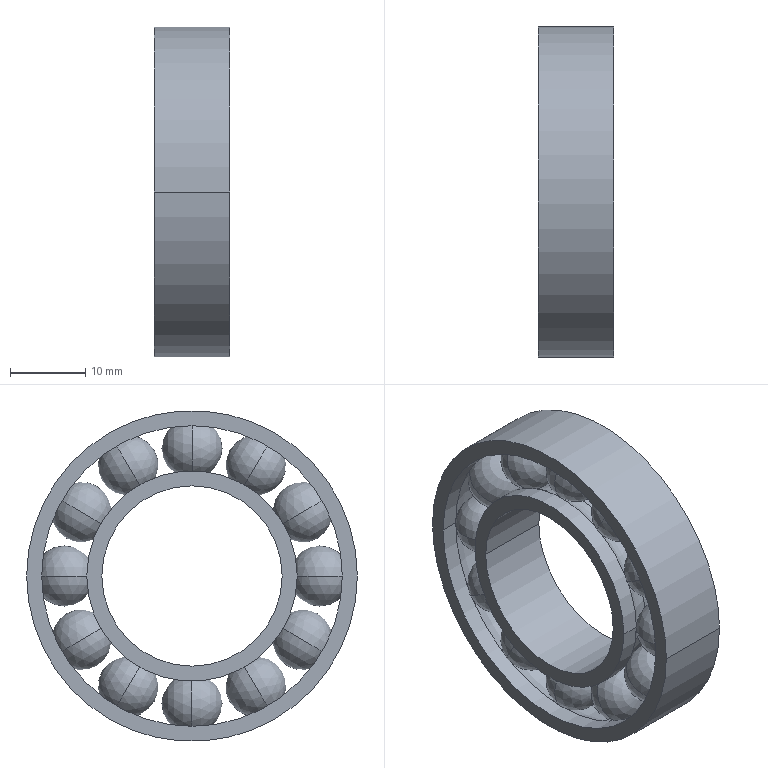Part | SolidWorks | features SavedExtBody 14 | 14 solids | 46 faces | box 10 x 44 x 44 mm | volume 6715 mm3 | sphere 24 | cylinder 12 | torus 6 | plane 4 | commonest cylinder face diameters 28 x4 40 x4 24 x2 44 x2
STEP:
#1=CARTESIAN_POINT('',(-83.272,6.5,53.742));
#2=VERTEX_POINT('',#1);
#3=CARTESIAN_POINT('',(-83.272,10.5,46.813));
#4=VERTEX_POINT('',#3);
#5=CARTESIAN_POINT('',(-83.272,8.5,50.278));
#6=DIRECTION('',(0.,0.866,0.5));
#7=DIRECTION('',(0.,-0.5,0.866));
#8=AXIS2_PLACEMENT_3D('',#5,#6,#7);
#9=CIRCLE('',#8,4.);
#10=EDGE_CURVE('',#2,#4,#9,.T.);
#11=ORIENTED_EDGE('',*,*,#10,.F.);
#12=CARTESIAN_POINT('',(-83.272,8.5,50.278));
#13=DIRECTION('',(0.,-0.866,-0.5));
#14=DIRECTION('',(0.,0.5,-0.866));
#15=AXIS2_PLACEMENT_3D('',#12,#13,#14);
#16=CIRCLE('',#15,4.);
#17=EDGE_CURVE('',#2,#4,#16,.T.);
#18=ORIENTED_EDGE('',*,*,#17,.T.);
#19=EDGE_LOOP('',(#11,#18));
#20=FACE_OUTER_BOUND('',#19,.T.);
#21=CARTESIAN_POINT('',(-83.272,8.5,50.278));
#22=DIRECTION('',(0.,-0.866,-0.5));
#23=DIRECTION('',(1.,0.,0.));
#24=AXIS2_PLACEMENT_3D('',#21,#22,#23);
#25=SPHERICAL_SURFACE('',#24,4.);
#26=ADVANCED_FACE('',(#20),#25,.T.);
#27=ORIENTED_EDGE('',*,*,#17,.F.);
#28=ORIENTED_EDGE('',*,*,#10,.T.);
#29=EDGE_LOOP('',(#27,#28));
#30=FACE_OUTER_BOUND('',#29,.T.);
#31=CARTESIAN_POINT('',(-83.272,8.5,50.278));
#32=DIRECTION('',(0.,-0.866,-0.5));
#33=DIRECTION('',(1.,0.,0.));
#34=AXIS2_PLACEMENT_3D('',#31,#32,#33);
#35=SPHERICAL_SURFACE('',#34,4.);
#36=ADVANCED_FACE('',(#30),#35,.T.);
#37=CLOSED_SHELL('',(#26,#36));
#38=MANIFOLD_SOLID_BREP('',#37);
#39=CARTESIAN_POINT('',(-83.272,11.258,58.5));
#40=VERTEX_POINT('',#39);
#41=CARTESIAN_POINT('',(-83.272,18.187,54.5));
#42=VERTEX_POINT('',#41);
#43=CARTESIAN_POINT('',(-83.272,14.722,56.5));
#44=DIRECTION('',(0.,0.5,0.866));
#45=DIRECTION('',(0.,-0.866,0.5));
#46=AXIS2_PLACEMENT_3D('',#43,#44,#45);
#47=CIRCLE('',#46,4.);
#48=EDGE_CURVE('',#40,#42,#47,.T.);
#49=ORIENTED_EDGE('',*,*,#48,.F.);
#50=CARTESIAN_POINT('',(-83.272,14.722,56.5));
#51=DIRECTION('',(0.,-0.5,-0.866));
#52=DIRECTION('',(0.,0.866,-0.5));
#53=AXIS2_PLACEMENT_3D('',#50,#51,#52);
#54=CIRCLE('',#53,4.);
#55=EDGE_CURVE('',#40,#42,#54,.T.);
#56=ORIENTED_EDGE('',*,*,#55,.T.);
#57=EDGE_LOOP('',(#49,#56));
#58=FACE_OUTER_BOUND('',#57,.T.);
#59=CARTESIAN_POINT('',(-83.272,14.722,56.5));
#60=DIRECTION('',(0.,-0.5,-0.866));
#61=DIRECTION('',(1.,0.,0.));
#62=AXIS2_PLACEMENT_3D('',#59,#60,#61);
#63=SPHERICAL_SURFACE('',#62,4.);
#64=ADVANCED_FACE('',(#58),#63,.T.);
#65=ORIENTED_EDGE('',*,*,#55,.F.);
#66=ORIENTED_EDGE('',*,*,#48,.T.);
#67=EDGE_LOOP('',(#65,#66));
#68=FACE_OUTER_BOUND('',#67,.T.);
#69=CARTESIAN_POINT('',(-83.272,14.722,56.5));
#70=DIRECTION('',(0.,-0.5,-0.866));
#71=DIRECTION('',(1.,0.,0.));
#72=AXIS2_PLACEMENT_3D('',#69,#70,#71);
#73=SPHERICAL_SURFACE('',#72,4.);
#74=ADVANCED_FACE('',(#68),#73,.T.);
#75=CLOSED_SHELL('',(#64,#74));
#76=MANIFOLD_SOLID_BREP('',#75);
#77=CARTESIAN_POINT('',(-83.272,13.,65.));
#78=VERTEX_POINT('',#77);
#79=CARTESIAN_POINT('',(-83.272,21.,65.));
#80=VERTEX_POINT('',#79);
#81=CARTESIAN_POINT('',(-83.272,17.,65.));
#82=DIRECTION('',(0.,0.,1.));
#83=DIRECTION('',(1.,0.,0.));
#84=AXIS2_PLACEMENT_3D('',#81,#82,#83);
#85=CIRCLE('',#84,4.);
#86=EDGE_CURVE('',#78,#80,#85,.T.);
#87=ORIENTED_EDGE('',*,*,#86,.F.);
#88=CARTESIAN_POINT('',(-83.272,17.,65.));
#89=DIRECTION('',(0.,0.,-1.));
#90=DIRECTION('',(-1.,0.,0.));
#91=AXIS2_PLACEMENT_3D('',#88,#89,#90);
#92=CIRCLE('',#91,4.);
#93=EDGE_CURVE('',#78,#80,#92,.T.);
#94=ORIENTED_EDGE('',*,*,#93,.T.);
#95=EDGE_LOOP('',(#87,#94));
#96=FACE_OUTER_BOUND('',#95,.T.);
#97=CARTESIAN_POINT('',(-83.272,17.,65.));
#98=DIRECTION('',(0.,0.,-1.));
#99=DIRECTION('',(1.,0.,0.));
#100=AXIS2_PLACEMENT_3D('',#97,#98,#99);
#101=SPHERICAL_SURFACE('',#100,4.);
#102=ADVANCED_FACE('',(#96),#101,.T.);
#103=ORIENTED_EDGE('',*,*,#93,.F.);
#104=ORIENTED_EDGE('',*,*,#86,.T.);
#105=EDGE_LOOP('',(#103,#104));
#106=FACE_OUTER_BOUND('',#105,.T.);
#107=CARTESIAN_POINT('',(-83.272,17.,65.));
#108=DIRECTION('',(0.,0.,-1.));
#109=DIRECTION('',(1.,0.,0.));
#110=AXIS2_PLACEMENT_3D('',#107,#108,#109);
#111=SPHERICAL_SURFACE('',#110,4.);
#112=ADVANCED_FACE('',(#106),#111,.T.);
#113=CLOSED_SHELL('',(#102,#112));
#114=MANIFOLD_SOLID_BREP('',#113);
#115=CARTESIAN_POINT('',(-83.272,11.258,71.5));
#116=VERTEX_POINT('',#115);
#117=CARTESIAN_POINT('',(-83.272,18.187,75.5));
#118=VERTEX_POINT('',#117);
#119=CARTESIAN_POINT('',(-83.272,14.722,73.5));
#120=DIRECTION('',(0.,-0.5,0.866));
#121=DIRECTION('',(0.,-0.866,-0.5));
#122=AXIS2_PLACEMENT_3D('',#119,#120,#121);
#123=CIRCLE('',#122,4.);
#124=EDGE_CURVE('',#116,#118,#123,.T.);
#125=ORIENTED_EDGE('',*,*,#124,.F.);
#126=CARTESIAN_POINT('',(-83.272,14.722,73.5));
#127=DIRECTION('',(0.,0.5,-0.866));
#128=DIRECTION('',(0.,0.866,0.5));
#129=AXIS2_PLACEMENT_3D('',#126,#127,#128);
#130=CIRCLE('',#129,4.);
#131=EDGE_CURVE('',#116,#118,#130,.T.);
#132=ORIENTED_EDGE('',*,*,#131,.T.);
#133=EDGE_LOOP('',(#125,#132));
#134=FACE_OUTER_BOUND('',#133,.T.);
#135=CARTESIAN_POINT('',(-83.272,14.722,73.5));
#136=DIRECTION('',(0.,0.5,-0.866));
#137=DIRECTION('',(1.,0.,0.));
#138=AXIS2_PLACEMENT_3D('',#135,#136,#137);
#139=SPHERICAL_SURFACE('',#138,4.);
#140=ADVANCED_FACE('',(#134),#139,.T.);
#141=ORIENTED_EDGE('',*,*,#131,.F.);
#142=ORIENTED_EDGE('',*,*,#124,.T.);
#143=EDGE_LOOP('',(#141,#142));
#144=FACE_OUTER_BOUND('',#143,.T.);
#145=CARTESIAN_POINT('',(-83.272,14.722,73.5));
#146=DIRECTION('',(0.,0.5,-0.866));
#147=DIRECTION('',(1.,0.,0.));
#148=AXIS2_PLACEMENT_3D('',#145,#146,#147);
#149=SPHERICAL_SURFACE('',#148,4.);
#150=ADVANCED_FACE('',(#144),#149,.T.);
#151=CLOSED_SHELL('',(#140,#150));
#152=MANIFOLD_SOLID_BREP('',#151);
#153=CARTESIAN_POINT('',(-83.272,6.5,76.258));
#154=VERTEX_POINT('',#153);
#155=CARTESIAN_POINT('',(-83.272,10.5,83.187));
#156=VERTEX_POINT('',#155);
#157=CARTESIAN_POINT('',(-83.272,8.5,79.722));
#158=DIRECTION('',(0.,-0.866,0.5));
#159=DIRECTION('',(0.,-0.5,-0.866));
#160=AXIS2_PLACEMENT_3D('',#157,#158,#159);
#161=CIRCLE('',#160,4.);
#162=EDGE_CURVE('',#154,#156,#161,.T.);
#163=ORIENTED_EDGE('',*,*,#162,.F.);
#164=CARTESIAN_POINT('',(-83.272,8.5,79.722));
#165=DIRECTION('',(0.,0.866,-0.5));
#166=DIRECTION('',(0.,0.5,0.866));
#167=AXIS2_PLACEMENT_3D('',#164,#165,#166);
#168=CIRCLE('',#167,4.);
#169=EDGE_CURVE('',#154,#156,#168,.T.);
#170=ORIENTED_EDGE('',*,*,#169,.T.);
#171=EDGE_LOOP('',(#163,#170));
#172=FACE_OUTER_BOUND('',#171,.T.);
#173=CARTESIAN_POINT('',(-83.272,8.5,79.722));
#174=DIRECTION('',(0.,0.866,-0.5));
#175=DIRECTION('',(1.,0.,0.));
#176=AXIS2_PLACEMENT_3D('',#173,#174,#175);
#177=SPHERICAL_SURFACE('',#176,4.);
#178=ADVANCED_FACE('',(#172),#177,.T.);
#179=ORIENTED_EDGE('',*,*,#169,.F.);
#180=ORIENTED_EDGE('',*,*,#162,.T.);
#181=EDGE_LOOP('',(#179,#180));
#182=FACE_OUTER_BOUND('',#181,.T.);
#183=CARTESIAN_POINT('',(-83.272,8.5,79.722));
#184=DIRECTION('',(0.,0.866,-0.5));
#185=DIRECTION('',(1.,0.,0.));
#186=AXIS2_PLACEMENT_3D('',#183,#184,#185);
#187=SPHERICAL_SURFACE('',#186,4.);
#188=ADVANCED_FACE('',(#182),#187,.T.);
#189=CLOSED_SHELL('',(#178,#188));
#190=MANIFOLD_SOLID_BREP('',#189);
#191=CARTESIAN_POINT('',(-83.272,0.,78.));
#192=VERTEX_POINT('',#191);
#193=CARTESIAN_POINT('',(-83.272,0.,86.));
#194=VERTEX_POINT('',#193);
#195=CARTESIAN_POINT('',(-83.272,0.,82.));
#196=DIRECTION('',(0.,-1.,0.));
#197=DIRECTION('',(0.,0.,-1.));
#198=AXIS2_PLACEMENT_3D('',#195,#196,#197);
#199=CIRCLE('',#198,4.);
#200=EDGE_CURVE('',#192,#194,#199,.T.);
#201=ORIENTED_EDGE('',*,*,#200,.F.);
#202=CARTESIAN_POINT('',(-83.272,0.,82.));
#203=DIRECTION('',(0.,1.,0.));
#204=DIRECTION('',(0.,0.,1.));
#205=AXIS2_PLACEMENT_3D('',#202,#203,#204);
#206=CIRCLE('',#205,4.);
#207=EDGE_CURVE('',#192,#194,#206,.T.);
#208=ORIENTED_EDGE('',*,*,#207,.T.);
#209=EDGE_LOOP('',(#201,#208));
#210=FACE_OUTER_BOUND('',#209,.T.);
#211=CARTESIAN_POINT('',(-83.272,0.,82.));
#212=DIRECTION('',(0.,1.,0.));
#213=DIRECTION('',(1.,0.,0.));
#214=AXIS2_PLACEMENT_3D('',#211,#212,#213);
#215=SPHERICAL_SURFACE('',#214,4.);
#216=ADVANCED_FACE('',(#210),#215,.T.);
#217=ORIENTED_EDGE('',*,*,#207,.F.);
#218=ORIENTED_EDGE('',*,*,#200,.T.);
#219=EDGE_LOOP('',(#217,#218));
#220=FACE_OUTER_BOUND('',#219,.T.);
#221=CARTESIAN_POINT('',(-83.272,0.,82.));
#222=DIRECTION('',(0.,1.,0.));
#223=DIRECTION('',(1.,0.,0.));
#224=AXIS2_PLACEMENT_3D('',#221,#222,#223);
#225=SPHERICAL_SURFACE('',#224,4.);
#226=ADVANCED_FACE('',(#220),#225,.T.);
#227=CLOSED_SHELL('',(#216,#226));
#228=MANIFOLD_SOLID_BREP('',#227);
#229=CARTESIAN_POINT('',(-83.272,-6.5,76.258));
#230=VERTEX_POINT('',#229);
#231=CARTESIAN_POINT('',(-83.272,-10.5,83.187));
#232=VERTEX_POINT('',#231);
#233=CARTESIAN_POINT('',(-83.272,-8.5,79.722));
#234=DIRECTION('',(0.,-0.866,-0.5));
#235=DIRECTION('',(0.,0.5,-0.866));
#236=AXIS2_PLACEMENT_3D('',#233,#234,#235);
#237=CIRCLE('',#236,4.);
#238=EDGE_CURVE('',#230,#232,#237,.T.);
#239=ORIENTED_EDGE('',*,*,#238,.F.);
#240=CARTESIAN_POINT('',(-83.272,-8.5,79.722));
#241=DIRECTION('',(0.,0.866,0.5));
#242=DIRECTION('',(0.,-0.5,0.866));
#243=AXIS2_PLACEMENT_3D('',#240,#241,#242);
#244=CIRCLE('',#243,4.);
#245=EDGE_CURVE('',#230,#232,#244,.T.);
#246=ORIENTED_EDGE('',*,*,#245,.T.);
#247=EDGE_LOOP('',(#239,#246));
#248=FACE_OUTER_BOUND('',#247,.T.);
#249=CARTESIAN_POINT('',(-83.272,-8.5,79.722));
#250=DIRECTION('',(0.,0.866,0.5));
#251=DIRECTION('',(1.,0.,0.));
#252=AXIS2_PLACEMENT_3D('',#249,#250,#251);
#253=SPHERICAL_SURFACE('',#252,4.);
#254=ADVANCED_FACE('',(#248),#253,.T.);
#255=ORIENTED_EDGE('',*,*,#245,.F.);
#256=ORIENTED_EDGE('',*,*,#238,.T.);
#257=EDGE_LOOP('',(#255,#256));
#258=FACE_OUTER_BOUND('',#257,.T.);
#259=CARTESIAN_POINT('',(-83.272,-8.5,79.722));
#260=DIRECTION('',(0.,0.866,0.5));
#261=DIRECTION('',(1.,0.,0.));
#262=AXIS2_PLACEMENT_3D('',#259,#260,#261);
#263=SPHERICAL_SURFACE('',#262,4.);
#264=ADVANCED_FACE('',(#258),#263,.T.);
#265=CLOSED_SHELL('',(#254,#264));
#266=MANIFOLD_SOLID_BREP('',#265);
#267=CARTESIAN_POINT('',(-83.272,-11.258,71.5));
#268=VERTEX_POINT('',#267);
#269=CARTESIAN_POINT('',(-83.272,-18.187,75.5));
#270=VERTEX_POINT('',#269);
#271=CARTESIAN_POINT('',(-83.272,-14.722,73.5));
#272=DIRECTION('',(0.,-0.5,-0.866));
#273=DIRECTION('',(0.,0.866,-0.5));
#274=AXIS2_PLACEMENT_3D('',#271,#272,#273);
#275=CIRCLE('',#274,4.);
#276=EDGE_CURVE('',#268,#270,#275,.T.);
#277=ORIENTED_EDGE('',*,*,#276,.F.);
#278=CARTESIAN_POINT('',(-83.272,-14.722,73.5));
#279=DIRECTION('',(0.,0.5,0.866));
#280=DIRECTION('',(0.,-0.866,0.5));
#281=AXIS2_PLACEMENT_3D('',#278,#279,#280);
#282=CIRCLE('',#281,4.);
#283=EDGE_CURVE('',#268,#270,#282,.T.);
#284=ORIENTED_EDGE('',*,*,#283,.T.);
#285=EDGE_LOOP('',(#277,#284));
#286=FACE_OUTER_BOUND('',#285,.T.);
#287=CARTESIAN_POINT('',(-83.272,-14.722,73.5));
#288=DIRECTION('',(0.,0.5,0.866));
#289=DIRECTION('',(1.,0.,0.));
#290=AXIS2_PLACEMENT_3D('',#287,#288,#289);
#291=SPHERICAL_SURFACE('',#290,4.);
#292=ADVANCED_FACE('',(#286),#291,.T.);
#293=ORIENTED_EDGE('',*,*,#283,.F.);
#294=ORIENTED_EDGE('',*,*,#276,.T.);
#295=EDGE_LOOP('',(#293,#294));
#296=FACE_OUTER_BOUND('',#295,.T.);
#297=CARTESIAN_POINT('',(-83.272,-14.722,73.5));
#298=DIRECTION('',(0.,0.5,0.866));
#299=DIRECTION('',(1.,0.,0.));
#300=AXIS2_PLACEMENT_3D('',#297,#298,#299);
#301=SPHERICAL_SURFACE('',#300,4.);
#302=ADVANCED_FACE('',(#296),#301,.T.);
#303=CLOSED_SHELL('',(#292,#302));
#304=MANIFOLD_SOLID_BREP('',#303);
#305=CARTESIAN_POINT('',(-83.272,-13.,65.));
#306=VERTEX_POINT('',#305);
#307=CARTESIAN_POINT('',(-83.272,-21.,65.));
#308=VERTEX_POINT('',#307);
#309=CARTESIAN_POINT('',(-83.272,-17.,65.));
#310=DIRECTION('',(0.,0.,-1.));
#311=DIRECTION('',(-1.,0.,0.));
#312=AXIS2_PLACEMENT_3D('',#309,#310,#311);
#313=CIRCLE('',#312,4.);
#314=EDGE_CURVE('',#306,#308,#313,.T.);
#315=ORIENTED_EDGE('',*,*,#314,.F.);
#316=CARTESIAN_POINT('',(-83.272,-17.,65.));
#317=DIRECTION('',(0.,0.,1.));
#318=DIRECTION('',(1.,0.,0.));
#319=AXIS2_PLACEMENT_3D('',#316,#317,#318);
#320=CIRCLE('',#319,4.);
#321=EDGE_CURVE('',#306,#308,#320,.T.);
#322=ORIENTED_EDGE('',*,*,#321,.T.);
#323=EDGE_LOOP('',(#315,#322));
#324=FACE_OUTER_BOUND('',#323,.T.);
#325=CARTESIAN_POINT('',(-83.272,-17.,65.));
#326=DIRECTION('',(0.,0.,1.));
#327=DIRECTION('',(1.,0.,0.));
#328=AXIS2_PLACEMENT_3D('',#325,#326,#327);
#329=SPHERICAL_SURFACE('',#328,4.);
#330=ADVANCED_FACE('',(#324),#329,.T.);
#331=ORIENTED_EDGE('',*,*,#321,.F.);
#332=ORIENTED_EDGE('',*,*,#314,.T.);
#333=EDGE_LOOP('',(#331,#332));
#334=FACE_OUTER_BOUND('',#333,.T.);
#335=CARTESIAN_POINT('',(-83.272,-17.,65.));
#336=DIRECTION('',(0.,0.,1.));
#337=DIRECTION('',(1.,0.,0.));
#338=AXIS2_PLACEMENT_3D('',#335,#336,#337);
#339=SPHERICAL_SURFACE('',#338,4.);
#340=ADVANCED_FACE('',(#334),#339,.T.);
#341=CLOSED_SHELL('',(#330,#340));
#342=MANIFOLD_SOLID_BREP('',#341);
#343=CARTESIAN_POINT('',(-83.272,-11.258,58.5));
#344=VERTEX_POINT('',#343);
#345=CARTESIAN_POINT('',(-83.272,-18.187,54.5));
#346=VERTEX_POINT('',#345);
#347=CARTESIAN_POINT('',(-83.272,-14.722,56.5));
#348=DIRECTION('',(0.,0.5,-0.866));
#349=DIRECTION('',(0.,0.866,0.5));
#350=AXIS2_PLACEMENT_3D('',#347,#348,#349);
#351=CIRCLE('',#350,4.);
#352=EDGE_CURVE('',#344,#346,#351,.T.);
#353=ORIENTED_EDGE('',*,*,#352,.F.);
#354=CARTESIAN_POINT('',(-83.272,-14.722,56.5));
#355=DIRECTION('',(0.,-0.5,0.866));
#356=DIRECTION('',(0.,-0.866,-0.5));
#357=AXIS2_PLACEMENT_3D('',#354,#355,#356);
#358=CIRCLE('',#357,4.);
#359=EDGE_CURVE('',#344,#346,#358,.T.);
#360=ORIENTED_EDGE('',*,*,#359,.T.);
#361=EDGE_LOOP('',(#353,#360));
#362=FACE_OUTER_BOUND('',#361,.T.);
#363=CARTESIAN_POINT('',(-83.272,-14.722,56.5));
#364=DIRECTION('',(0.,-0.5,0.866));
#365=DIRECTION('',(1.,0.,0.));
#366=AXIS2_PLACEMENT_3D('',#363,#364,#365);
#367=SPHERICAL_SURFACE('',#366,4.);
#368=ADVANCED_FACE('',(#362),#367,.T.);
#369=ORIENTED_EDGE('',*,*,#359,.F.);
#370=ORIENTED_EDGE('',*,*,#352,.T.);
#371=EDGE_LOOP('',(#369,#370));
#372=FACE_OUTER_BOUND('',#371,.T.);
#373=CARTESIAN_POINT('',(-83.272,-14.722,56.5));
#374=DIRECTION('',(0.,-0.5,0.866));
#375=DIRECTION('',(1.,0.,0.));
#376=AXIS2_PLACEMENT_3D('',#373,#374,#375);
#377=SPHERICAL_SURFACE('',#376,4.);
#378=ADVANCED_FACE('',(#372),#377,.T.);
#379=CLOSED_SHELL('',(#368,#378));
#380=MANIFOLD_SOLID_BREP('',#379);
#381=CARTESIAN_POINT('',(-83.272,-6.5,53.742));
#382=VERTEX_POINT('',#381);
#383=CARTESIAN_POINT('',(-83.272,-10.5,46.813));
#384=VERTEX_POINT('',#383);
#385=CARTESIAN_POINT('',(-83.272,-8.5,50.278));
#386=DIRECTION('',(0.,0.866,-0.5));
#387=DIRECTION('',(0.,0.5,0.866));
#388=AXIS2_PLACEMENT_3D('',#385,#386,#387);
#389=CIRCLE('',#388,4.);
#390=EDGE_CURVE('',#382,#384,#389,.T.);
#391=ORIENTED_EDGE('',*,*,#390,.F.);
#392=CARTESIAN_POINT('',(-83.272,-8.5,50.278));
#393=DIRECTION('',(0.,-0.866,0.5));
#394=DIRECTION('',(0.,-0.5,-0.866));
#395=AXIS2_PLACEMENT_3D('',#392,#393,#394);
#396=CIRCLE('',#395,4.);
#397=EDGE_CURVE('',#382,#384,#396,.T.);
#398=ORIENTED_EDGE('',*,*,#397,.T.);
#399=EDGE_LOOP('',(#391,#398));
#400=FACE_OUTER_BOUND('',#399,.T.);
#401=CARTESIAN_POINT('',(-83.272,-8.5,50.278));
#402=DIRECTION('',(0.,-0.866,0.5));
#403=DIRECTION('',(1.,0.,0.));
#404=AXIS2_PLACEMENT_3D('',#401,#402,#403);
#405=SPHERICAL_SURFACE('',#404,4.);
#406=ADVANCED_FACE('',(#400),#405,.T.);
#407=ORIENTED_EDGE('',*,*,#397,.F.);
#408=ORIENTED_EDGE('',*,*,#390,.T.);
#409=EDGE_LOOP('',(#407,#408));
#410=FACE_OUTER_BOUND('',#409,.T.);
#411=CARTESIAN_POINT('',(-83.272,-8.5,50.278));
#412=DIRECTION('',(0.,-0.866,0.5));
#413=DIRECTION('',(1.,0.,0.));
#414=AXIS2_PLACEMENT_3D('',#411,#412,#413);
#415=SPHERICAL_SURFACE('',#414,4.);
#416=ADVANCED_FACE('',(#410),#415,.T.);
#417=CLOSED_SHELL('',(#406,#416));
#418=MANIFOLD_SOLID_BREP('',#417);
#419=CARTESIAN_POINT('',(-83.272,0.,52.));
#420=VERTEX_POINT('',#419);
#421=CARTESIAN_POINT('',(-83.272,0.,44.));
#422=VERTEX_POINT('',#421);
#423=CARTESIAN_POINT('',(-83.272,0.,48.));
#424=DIRECTION('',(0.,1.,0.));
#425=DIRECTION('',(0.,0.,1.));
#426=AXIS2_PLACEMENT_3D('',#423,#424,#425);
#427=CIRCLE('',#426,4.);
#428=EDGE_CURVE('',#420,#422,#427,.T.);
#429=ORIENTED_EDGE('',*,*,#428,.F.);
#430=CARTESIAN_POINT('',(-83.272,0.,48.));
#431=DIRECTION('',(0.,-1.,0.));
#432=DIRECTION('',(0.,0.,-1.));
#433=AXIS2_PLACEMENT_3D('',#430,#431,#432);
#434=CIRCLE('',#433,4.);
#435=EDGE_CURVE('',#420,#422,#434,.T.);
#436=ORIENTED_EDGE('',*,*,#435,.T.);
#437=EDGE_LOOP('',(#429,#436));
#438=FACE_OUTER_BOUND('',#437,.T.);
#439=CARTESIAN_POINT('',(-83.272,0.,48.));
#440=DIRECTION('',(0.,-1.,0.));
#441=DIRECTION('',(1.,0.,0.));
#442=AXIS2_PLACEMENT_3D('',#439,#440,#441);
#443=SPHERICAL_SURFACE('',#442,4.);
#444=ADVANCED_FACE('',(#438),#443,.T.);
#445=ORIENTED_EDGE('',*,*,#435,.F.);
#446=ORIENTED_EDGE('',*,*,#428,.T.);
#447=EDGE_LOOP('',(#445,#446));
#448=FACE_OUTER_BOUND('',#447,.T.);
#449=CARTESIAN_POINT('',(-83.272,0.,48.));
#450=DIRECTION('',(0.,-1.,0.));
#451=DIRECTION('',(1.,0.,0.));
#452=AXIS2_PLACEMENT_3D('',#449,#450,#451);
#453=SPHERICAL_SURFACE('',#452,4.);
#454=ADVANCED_FACE('',(#448),#453,.T.);
#455=CLOSED_SHELL('',(#444,#454));
#456=MANIFOLD_SOLID_BREP('',#455);
#457=CARTESIAN_POINT('',(-80.627,20.,65.));
#458=VERTEX_POINT('',#457);
#459=CARTESIAN_POINT('',(-80.627,-20.,65.));
#460=VERTEX_POINT('',#459);
#461=CARTESIAN_POINT('',(-80.627,0.,65.));
#462=DIRECTION('',(-1.,0.,0.));
#463=DIRECTION('',(0.,-1.,0.));
#464=AXIS2_PLACEMENT_3D('',#461,#462,#463);
#465=CIRCLE('',#464,20.);
#466=EDGE_CURVE('',#458,#460,#465,.T.);
#467=ORIENTED_EDGE('',*,*,#466,.F.);
#468=CARTESIAN_POINT('',(-85.918,20.,65.));
#469=VERTEX_POINT('',#468);
#470=CARTESIAN_POINT('',(-83.272,17.,65.));
#471=DIRECTION('',(0.,0.,1.));
#472=DIRECTION('',(0.,-1.,0.));
#473=AXIS2_PLACEMENT_3D('',#470,#471,#472);
#474=CIRCLE('',#473,4.);
#475=EDGE_CURVE('',#458,#469,#474,.T.);
#476=ORIENTED_EDGE('',*,*,#475,.T.);
#477=CARTESIAN_POINT('',(-85.918,-20.,65.));
#478=VERTEX_POINT('',#477);
#479=CARTESIAN_POINT('',(-85.918,0.,65.));
#480=DIRECTION('',(1.,0.,0.));
#481=DIRECTION('',(0.,1.,0.));
#482=AXIS2_PLACEMENT_3D('',#479,#480,#481);
#483=CIRCLE('',#482,20.);
#484=EDGE_CURVE('',#478,#469,#483,.T.);
#485=ORIENTED_EDGE('',*,*,#484,.F.);
#486=CARTESIAN_POINT('',(-83.272,-17.,65.));
#487=DIRECTION('',(0.,0.,-1.));
#488=DIRECTION('',(-1.,0.,0.));
#489=AXIS2_PLACEMENT_3D('',#486,#487,#488);
#490=CIRCLE('',#489,4.);
#491=EDGE_CURVE('',#460,#478,#490,.T.);
#492=ORIENTED_EDGE('',*,*,#491,.F.);
#493=EDGE_LOOP('',(#467,#476,#485,#492));
#494=FACE_OUTER_BOUND('',#493,.T.);
#495=CARTESIAN_POINT('',(-83.272,0.,65.));
#496=DIRECTION('',(-1.,0.,0.));
#497=DIRECTION('',(0.,-1.,0.));
#498=AXIS2_PLACEMENT_3D('',#495,#496,#497);
#499=TOROIDAL_SURFACE('',#498,17.,4.);
#500=ADVANCED_FACE('',(#494),#499,.F.);
#501=CARTESIAN_POINT('',(-88.272,-22.,65.));
#502=VERTEX_POINT('',#501);
#503=CARTESIAN_POINT('',(-88.272,22.,65.));
#504=VERTEX_POINT('',#503);
#505=CARTESIAN_POINT('',(-88.272,0.,65.));
#506=DIRECTION('',(-1.,0.,0.));
#507=DIRECTION('',(0.,0.,1.));
#508=AXIS2_PLACEMENT_3D('',#505,#506,#507);
#509=CIRCLE('',#508,22.);
#510=EDGE_CURVE('',#502,#504,#509,.T.);
#511=ORIENTED_EDGE('',*,*,#510,.F.);
#512=CARTESIAN_POINT('',(-78.272,-22.,65.));
#513=VERTEX_POINT('',#512);
#514=CARTESIAN_POINT('',(-150.498,-22.,65.));
#515=DIRECTION('',(1.,0.,0.));
#516=VECTOR('',#515,1000.);
#517=LINE('',#514,#516);
#518=EDGE_CURVE('',#502,#513,#517,.T.);
#519=ORIENTED_EDGE('',*,*,#518,.T.);
#520=CARTESIAN_POINT('',(-78.272,22.,65.));
#521=VERTEX_POINT('',#520);
#522=CARTESIAN_POINT('',(-78.272,0.,65.));
#523=DIRECTION('',(-1.,0.,0.));
#524=DIRECTION('',(0.,0.,1.));
#525=AXIS2_PLACEMENT_3D('',#522,#523,#524);
#526=CIRCLE('',#525,22.);
#527=EDGE_CURVE('',#513,#521,#526,.T.);
#528=ORIENTED_EDGE('',*,*,#527,.T.);
#529=CARTESIAN_POINT('',(-150.498,22.,65.));
#530=DIRECTION('',(1.,0.,0.));
#531=VECTOR('',#530,1000.);
#532=LINE('',#529,#531);
#533=EDGE_CURVE('',#504,#521,#532,.T.);
#534=ORIENTED_EDGE('',*,*,#533,.F.);
#535=EDGE_LOOP('',(#511,#519,#528,#534));
#536=FACE_OUTER_BOUND('',#535,.T.);
#537=CARTESIAN_POINT('',(-150.498,0.,65.));
#538=DIRECTION('',(1.,0.,0.));
#539=DIRECTION('',(0.,1.,0.));
#540=AXIS2_PLACEMENT_3D('',#537,#538,#539);
#541=CYLINDRICAL_SURFACE('',#540,22.);
#542=ADVANCED_FACE('',(#536),#541,.T.);
#543=ORIENTED_EDGE('',*,*,#466,.T.);
#544=CARTESIAN_POINT('',(-78.272,-20.,65.));
#545=VERTEX_POINT('',#544);
#546=CARTESIAN_POINT('',(-150.498,-20.,65.));
#547=DIRECTION('',(1.,0.,0.));
#548=VECTOR('',#547,1000.);
#549=LINE('',#546,#548);
#550=EDGE_CURVE('',#460,#545,#549,.T.);
#551=ORIENTED_EDGE('',*,*,#550,.T.);
#552=CARTESIAN_POINT('',(-78.272,20.,65.));
#553=VERTEX_POINT('',#552);
#554=CARTESIAN_POINT('',(-78.272,0.,65.));
#555=DIRECTION('',(-1.,0.,0.));
#556=DIRECTION('',(0.,0.,1.));
#557=AXIS2_PLACEMENT_3D('',#554,#555,#556);
#558=CIRCLE('',#557,20.);
#559=EDGE_CURVE('',#553,#545,#558,.T.);
#560=ORIENTED_EDGE('',*,*,#559,.F.);
#561=CARTESIAN_POINT('',(-150.498,20.,65.));
#562=DIRECTION('',(1.,0.,0.));
#563=VECTOR('',#562,1000.);
#564=LINE('',#561,#563);
#565=EDGE_CURVE('',#458,#553,#564,.T.);
#566=ORIENTED_EDGE('',*,*,#565,.F.);
#567=EDGE_LOOP('',(#543,#551,#560,#566));
#568=FACE_OUTER_BOUND('',#567,.T.);
#569=CARTESIAN_POINT('',(-150.498,0.,65.));
#570=DIRECTION('',(1.,0.,0.));
#571=DIRECTION('',(0.,1.,0.));
#572=AXIS2_PLACEMENT_3D('',#569,#570,#571);
#573=CYLINDRICAL_SURFACE('',#572,20.);
#574=ADVANCED_FACE('',(#568),#573,.F.);
#575=CARTESIAN_POINT('',(-88.272,20.,65.));
#576=VERTEX_POINT('',#575);
#577=CARTESIAN_POINT('',(-88.272,-20.,65.));
#578=VERTEX_POINT('',#577);
#579=CARTESIAN_POINT('',(-88.272,0.,65.));
#580=DIRECTION('',(-1.,0.,0.));
#581=DIRECTION('',(0.,0.,1.));
#582=AXIS2_PLACEMENT_3D('',#579,#580,#581);
#583=CIRCLE('',#582,20.);
#584=EDGE_CURVE('',#576,#578,#583,.T.);
#585=ORIENTED_EDGE('',*,*,#584,.T.);
#586=CARTESIAN_POINT('',(-150.498,-20.,65.));
#587=DIRECTION('',(1.,0.,0.));
#588=VECTOR('',#587,1000.);
#589=LINE('',#586,#588);
#590=EDGE_CURVE('',#578,#478,#589,.T.);
#591=ORIENTED_EDGE('',*,*,#590,.T.);
#592=ORIENTED_EDGE('',*,*,#484,.T.);
#593=CARTESIAN_POINT('',(-150.498,20.,65.));
#594=DIRECTION('',(1.,0.,0.));
#595=VECTOR('',#594,1000.);
#596=LINE('',#593,#595);
#597=EDGE_CURVE('',#576,#469,#596,.T.);
#598=ORIENTED_EDGE('',*,*,#597,.F.);
#599=EDGE_LOOP('',(#585,#591,#592,#598));
#600=FACE_OUTER_BOUND('',#599,.T.);
#601=CARTESIAN_POINT('',(-150.498,0.,65.));
#602=DIRECTION('',(1.,0.,0.));
#603=DIRECTION('',(0.,1.,0.));
#604=AXIS2_PLACEMENT_3D('',#601,#602,#603);
#605=CYLINDRICAL_SURFACE('',#604,20.);
#606=ADVANCED_FACE('',(#600),#605,.F.);
#607=ORIENTED_EDGE('',*,*,#590,.F.);
#608=CARTESIAN_POINT('',(-88.272,0.,65.));
#609=DIRECTION('',(-1.,0.,0.));
#610=DIRECTION('',(0.,0.,1.));
#611=AXIS2_PLACEMENT_3D('',#608,#609,#610);
#612=CIRCLE('',#611,20.);
#613=EDGE_CURVE('',#578,#576,#612,.T.);
#614=ORIENTED_EDGE('',*,*,#613,.T.);
#615=ORIENTED_EDGE('',*,*,#597,.T.);
#616=CARTESIAN_POINT('',(-85.918,0.,65.));
#617=DIRECTION('',(1.,0.,0.));
#618=DIRECTION('',(0.,1.,0.));
#619=AXIS2_PLACEMENT_3D('',#616,#617,#618);
#620=CIRCLE('',#619,20.);
#621=EDGE_CURVE('',#469,#478,#620,.T.);
#622=ORIENTED_EDGE('',*,*,#621,.T.);
#623=EDGE_LOOP('',(#607,#614,#615,#622));
#624=FACE_OUTER_BOUND('',#623,.T.);
#625=CARTESIAN_POINT('',(-150.498,0.,65.));
#626=DIRECTION('',(1.,0.,0.));
#627=DIRECTION('',(0.,1.,0.));
#628=AXIS2_PLACEMENT_3D('',#625,#626,#627);
#629=CYLINDRICAL_SURFACE('',#628,20.);
#630=ADVANCED_FACE('',(#624),#629,.F.);
#631=ORIENTED_EDGE('',*,*,#550,.F.);
#632=CARTESIAN_POINT('',(-80.627,0.,65.));
#633=DIRECTION('',(-1.,0.,0.));
#634=DIRECTION('',(0.,-1.,0.));
#635=AXIS2_PLACEMENT_3D('',#632,#633,#634);
#636=CIRCLE('',#635,20.);
#637=EDGE_CURVE('',#460,#458,#636,.T.);
#638=ORIENTED_EDGE('',*,*,#637,.T.);
#639=ORIENTED_EDGE('',*,*,#565,.T.);
#640=CARTESIAN_POINT('',(-78.272,0.,65.));
#641=DIRECTION('',(-1.,0.,0.));
#642=DIRECTION('',(0.,0.,1.));
#643=AXIS2_PLACEMENT_3D('',#640,#641,#642);
#644=CIRCLE('',#643,20.);
#645=EDGE_CURVE('',#545,#553,#644,.T.);
#646=ORIENTED_EDGE('',*,*,#645,.F.);
#647=EDGE_LOOP('',(#631,#638,#639,#646));
#648=FACE_OUTER_BOUND('',#647,.T.);
#649=CARTESIAN_POINT('',(-150.498,0.,65.));
#650=DIRECTION('',(1.,0.,0.));
#651=DIRECTION('',(0.,1.,0.));
#652=AXIS2_PLACEMENT_3D('',#649,#650,#651);
#653=CYLINDRICAL_SURFACE('',#652,20.);
#654=ADVANCED_FACE('',(#648),#653,.F.);
#655=ORIENTED_EDGE('',*,*,#518,.F.);
#656=CARTESIAN_POINT('',(-88.272,0.,65.));
#657=DIRECTION('',(-1.,0.,0.));
#658=DIRECTION('',(0.,0.,1.));
#659=AXIS2_PLACEMENT_3D('',#656,#657,#658);
#660=CIRCLE('',#659,22.);
#661=EDGE_CURVE('',#504,#502,#660,.T.);
#662=ORIENTED_EDGE('',*,*,#661,.F.);
#663=ORIENTED_EDGE('',*,*,#533,.T.);
#664=CARTESIAN_POINT('',(-78.272,0.,65.));
#665=DIRECTION('',(-1.,0.,0.));
#666=DIRECTION('',(0.,0.,1.));
#667=AXIS2_PLACEMENT_3D('',#664,#665,#666);
#668=CIRCLE('',#667,22.);
#669=EDGE_CURVE('',#521,#513,#668,.T.);
#670=ORIENTED_EDGE('',*,*,#669,.T.);
#671=EDGE_LOOP('',(#655,#662,#663,#670));
#672=FACE_OUTER_BOUND('',#671,.T.);
#673=CARTESIAN_POINT('',(-150.498,0.,65.));
#674=DIRECTION('',(1.,0.,0.));
#675=DIRECTION('',(0.,1.,0.));
#676=AXIS2_PLACEMENT_3D('',#673,#674,#675);
#677=CYLINDRICAL_SURFACE('',#676,22.);
#678=ADVANCED_FACE('',(#672),#677,.T.);
#679=ORIENTED_EDGE('',*,*,#559,.T.);
#680=ORIENTED_EDGE('',*,*,#645,.T.);
#681=EDGE_LOOP('',(#679,#680));
#682=FACE_BOUND('',#681,.T.);
#683=ORIENTED_EDGE('',*,*,#669,.F.);
#684=ORIENTED_EDGE('',*,*,#527,.F.);
#685=EDGE_LOOP('',(#683,#684));
#686=FACE_OUTER_BOUND('',#685,.T.);
#687=CARTESIAN_POINT('',(-78.272,0.,0.));
#688=DIRECTION('',(-1.,0.,0.));
#689=DIRECTION('',(0.,0.,1.));
#690=AXIS2_PLACEMENT_3D('',#687,#688,#689);
#691=PLANE('',#690);
#692=ADVANCED_FACE('',(#682,#686),#691,.F.);
#693=ORIENTED_EDGE('',*,*,#584,.F.);
#694=ORIENTED_EDGE('',*,*,#613,.F.);
#695=EDGE_LOOP('',(#693,#694));
#696=FACE_BOUND('',#695,.T.);
#697=ORIENTED_EDGE('',*,*,#661,.T.);
#698=ORIENTED_EDGE('',*,*,#510,.T.);
#699=EDGE_LOOP('',(#697,#698));
#700=FACE_OUTER_BOUND('',#699,.T.);
#701=CARTESIAN_POINT('',(-88.272,0.,65.));
#702=DIRECTION('',(-1.,0.,0.));
#703=DIRECTION('',(0.,0.,1.));
#704=AXIS2_PLACEMENT_3D('',#701,#702,#703);
#705=PLANE('',#704);
#706=ADVANCED_FACE('',(#696,#700),#705,.T.);
#707=ORIENTED_EDGE('',*,*,#475,.F.);
#708=ORIENTED_EDGE('',*,*,#637,.F.);
#709=ORIENTED_EDGE('',*,*,#491,.T.);
#710=ORIENTED_EDGE('',*,*,#621,.F.);
#711=EDGE_LOOP('',(#707,#708,#709,#710));
#712=FACE_OUTER_BOUND('',#711,.T.);
#713=CARTESIAN_POINT('',(-83.272,0.,65.));
#714=DIRECTION('',(-1.,0.,0.));
#715=DIRECTION('',(0.,-1.,0.));
#716=AXIS2_PLACEMENT_3D('',#713,#714,#715);
#717=TOROIDAL_SURFACE('',#716,17.,4.);
#718=ADVANCED_FACE('',(#712),#717,.F.);
#719=CLOSED_SHELL('',(#500,#542,#574,#606,#630,#654,#678,#692,#706,#718));
#720=MANIFOLD_SOLID_BREP('',#719);
#721=CARTESIAN_POINT('',(-85.918,-14.,65.));
#722=VERTEX_POINT('',#721);
#723=CARTESIAN_POINT('',(-83.272,-13.,65.));
#724=VERTEX_POINT('',#723);
#725=CARTESIAN_POINT('',(-83.272,-17.,65.));
#726=DIRECTION('',(0.,0.,-1.));
#727=DIRECTION('',(-1.,0.,0.));
#728=AXIS2_PLACEMENT_3D('',#725,#726,#727);
#729=CIRCLE('',#728,4.);
#730=EDGE_CURVE('',#722,#724,#729,.T.);
#731=ORIENTED_EDGE('',*,*,#730,.T.);
#732=CARTESIAN_POINT('',(-83.272,13.,65.));
#733=VERTEX_POINT('',#732);
#734=CARTESIAN_POINT('',(-83.272,0.,65.));
#735=DIRECTION('',(-1.,0.,0.));
#736=DIRECTION('',(0.,-1.,0.));
#737=AXIS2_PLACEMENT_3D('',#734,#735,#736);
#738=CIRCLE('',#737,13.);
#739=EDGE_CURVE('',#724,#733,#738,.T.);
#740=ORIENTED_EDGE('',*,*,#739,.T.);
#741=CARTESIAN_POINT('',(-85.918,14.,65.));
#742=VERTEX_POINT('',#741);
#743=CARTESIAN_POINT('',(-83.272,17.,65.));
#744=DIRECTION('',(0.,0.,1.));
#745=DIRECTION('',(0.,-1.,0.));
#746=AXIS2_PLACEMENT_3D('',#743,#744,#745);
#747=CIRCLE('',#746,4.);
#748=EDGE_CURVE('',#742,#733,#747,.T.);
#749=ORIENTED_EDGE('',*,*,#748,.F.);
#750=CARTESIAN_POINT('',(-85.918,0.,65.));
#751=DIRECTION('',(1.,0.,0.));
#752=DIRECTION('',(0.,1.,0.));
#753=AXIS2_PLACEMENT_3D('',#750,#751,#752);
#754=CIRCLE('',#753,14.);
#755=EDGE_CURVE('',#742,#722,#754,.T.);
#756=ORIENTED_EDGE('',*,*,#755,.T.);
#757=EDGE_LOOP('',(#731,#740,#749,#756));
#758=FACE_OUTER_BOUND('',#757,.T.);
#759=CARTESIAN_POINT('',(-83.272,0.,65.));
#760=DIRECTION('',(-1.,0.,0.));
#761=DIRECTION('',(0.,-1.,0.));
#762=AXIS2_PLACEMENT_3D('',#759,#760,#761);
#763=TOROIDAL_SURFACE('',#762,17.,4.);
#764=ADVANCED_FACE('',(#758),#763,.F.);
#765=ORIENTED_EDGE('',*,*,#748,.T.);
#766=CARTESIAN_POINT('',(-83.272,0.,65.));
#767=DIRECTION('',(-1.,0.,0.));
#768=DIRECTION('',(0.,-1.,0.));
#769=AXIS2_PLACEMENT_3D('',#766,#767,#768);
#770=CIRCLE('',#769,13.);
#771=EDGE_CURVE('',#733,#724,#770,.T.);
#772=ORIENTED_EDGE('',*,*,#771,.T.);
#773=ORIENTED_EDGE('',*,*,#730,.F.);
#774=CARTESIAN_POINT('',(-85.918,0.,65.));
#775=DIRECTION('',(1.,0.,0.));
#776=DIRECTION('',(0.,1.,0.));
#777=AXIS2_PLACEMENT_3D('',#774,#775,#776);
#778=CIRCLE('',#777,14.);
#779=EDGE_CURVE('',#722,#742,#778,.T.);
#780=ORIENTED_EDGE('',*,*,#779,.T.);
#781=EDGE_LOOP('',(#765,#772,#773,#780));
#782=FACE_OUTER_BOUND('',#781,.T.);
#783=CARTESIAN_POINT('',(-83.272,0.,65.));
#784=DIRECTION('',(-1.,0.,0.));
#785=DIRECTION('',(0.,-1.,0.));
#786=AXIS2_PLACEMENT_3D('',#783,#784,#785);
#787=TOROIDAL_SURFACE('',#786,17.,4.);
#788=ADVANCED_FACE('',(#782),#787,.F.);
#789=ORIENTED_EDGE('',*,*,#771,.F.);
#790=CARTESIAN_POINT('',(-80.627,14.,65.));
#791=VERTEX_POINT('',#790);
#792=CARTESIAN_POINT('',(-83.272,17.,65.));
#793=DIRECTION('',(0.,0.,1.));
#794=DIRECTION('',(0.,-1.,0.));
#795=AXIS2_PLACEMENT_3D('',#792,#793,#794);
#796=CIRCLE('',#795,4.);
#797=EDGE_CURVE('',#733,#791,#796,.T.);
#798=ORIENTED_EDGE('',*,*,#797,.T.);
#799=CARTESIAN_POINT('',(-80.627,-14.,65.));
#800=VERTEX_POINT('',#799);
#801=CARTESIAN_POINT('',(-80.627,0.,65.));
#802=DIRECTION('',(-1.,0.,0.));
#803=DIRECTION('',(0.,-1.,0.));
#804=AXIS2_PLACEMENT_3D('',#801,#802,#803);
#805=CIRCLE('',#804,14.);
#806=EDGE_CURVE('',#791,#800,#805,.T.);
#807=ORIENTED_EDGE('',*,*,#806,.T.);
#808=CARTESIAN_POINT('',(-83.272,-17.,65.));
#809=DIRECTION('',(0.,0.,-1.));
#810=DIRECTION('',(-1.,0.,0.));
#811=AXIS2_PLACEMENT_3D('',#808,#809,#810);
#812=CIRCLE('',#811,4.);
#813=EDGE_CURVE('',#724,#800,#812,.T.);
#814=ORIENTED_EDGE('',*,*,#813,.F.);
#815=EDGE_LOOP('',(#789,#798,#807,#814));
#816=FACE_OUTER_BOUND('',#815,.T.);
#817=CARTESIAN_POINT('',(-83.272,0.,65.));
#818=DIRECTION('',(-1.,0.,0.));
#819=DIRECTION('',(0.,-1.,0.));
#820=AXIS2_PLACEMENT_3D('',#817,#818,#819);
#821=TOROIDAL_SURFACE('',#820,17.,4.);
#822=ADVANCED_FACE('',(#816),#821,.F.);
#823=CARTESIAN_POINT('',(-88.272,-12.,65.));
#824=VERTEX_POINT('',#823);
#825=CARTESIAN_POINT('',(-88.272,12.,65.));
#826=VERTEX_POINT('',#825);
#827=CARTESIAN_POINT('',(-88.272,0.,65.));
#828=DIRECTION('',(1.,0.,0.));
#829=DIRECTION('',(0.,0.,1.));
#830=AXIS2_PLACEMENT_3D('',#827,#828,#829);
#831=CIRCLE('',#830,12.);
#832=EDGE_CURVE('',#824,#826,#831,.T.);
#833=ORIENTED_EDGE('',*,*,#832,.F.);
#834=CARTESIAN_POINT('',(-78.272,-12.,65.));
#835=VERTEX_POINT('',#834);
#836=CARTESIAN_POINT('',(-150.498,-12.,65.));
#837=DIRECTION('',(1.,0.,0.));
#838=VECTOR('',#837,1000.);
#839=LINE('',#836,#838);
#840=EDGE_CURVE('',#824,#835,#839,.T.);
#841=ORIENTED_EDGE('',*,*,#840,.T.);
#842=CARTESIAN_POINT('',(-78.272,12.,65.));
#843=VERTEX_POINT('',#842);
#844=CARTESIAN_POINT('',(-78.272,0.,65.));
#845=DIRECTION('',(1.,0.,0.));
#846=DIRECTION('',(0.,0.,1.));
#847=AXIS2_PLACEMENT_3D('',#844,#845,#846);
#848=CIRCLE('',#847,12.);
#849=EDGE_CURVE('',#835,#843,#848,.T.);
#850=ORIENTED_EDGE('',*,*,#849,.T.);
#851=CARTESIAN_POINT('',(-150.498,12.,65.));
#852=DIRECTION('',(1.,0.,0.));
#853=VECTOR('',#852,1000.);
#854=LINE('',#851,#853);
#855=EDGE_CURVE('',#826,#843,#854,.T.);
#856=ORIENTED_EDGE('',*,*,#855,.F.);
#857=EDGE_LOOP('',(#833,#841,#850,#856));
#858=FACE_OUTER_BOUND('',#857,.T.);
#859=CARTESIAN_POINT('',(-150.498,0.,65.));
#860=DIRECTION('',(1.,0.,0.));
#861=DIRECTION('',(0.,1.,0.));
#862=AXIS2_PLACEMENT_3D('',#859,#860,#861);
#863=CYLINDRICAL_SURFACE('',#862,12.);
#864=ADVANCED_FACE('',(#858),#863,.F.);
#865=CARTESIAN_POINT('',(-80.627,0.,65.));
#866=DIRECTION('',(-1.,0.,0.));
#867=DIRECTION('',(0.,-1.,0.));
#868=AXIS2_PLACEMENT_3D('',#865,#866,#867);
#869=CIRCLE('',#868,14.);
#870=EDGE_CURVE('',#800,#791,#869,.T.);
#871=ORIENTED_EDGE('',*,*,#870,.F.);
#872=CARTESIAN_POINT('',(-78.272,-14.,65.));
#873=VERTEX_POINT('',#872);
#874=CARTESIAN_POINT('',(-150.498,-14.,65.));
#875=DIRECTION('',(1.,0.,0.));
#876=VECTOR('',#875,1000.);
#877=LINE('',#874,#876);
#878=EDGE_CURVE('',#800,#873,#877,.T.);
#879=ORIENTED_EDGE('',*,*,#878,.T.);
#880=CARTESIAN_POINT('',(-78.272,14.,65.));
#881=VERTEX_POINT('',#880);
#882=CARTESIAN_POINT('',(-78.272,0.,65.));
#883=DIRECTION('',(-1.,0.,0.));
#884=DIRECTION('',(0.,0.,1.));
#885=AXIS2_PLACEMENT_3D('',#882,#883,#884);
#886=CIRCLE('',#885,14.);
#887=EDGE_CURVE('',#873,#881,#886,.T.);
#888=ORIENTED_EDGE('',*,*,#887,.T.);
#889=CARTESIAN_POINT('',(-150.498,14.,65.));
#890=DIRECTION('',(1.,0.,0.));
#891=VECTOR('',#890,1000.);
#892=LINE('',#889,#891);
#893=EDGE_CURVE('',#791,#881,#892,.T.);
#894=ORIENTED_EDGE('',*,*,#893,.F.);
#895=EDGE_LOOP('',(#871,#879,#888,#894));
#896=FACE_OUTER_BOUND('',#895,.T.);
#897=CARTESIAN_POINT('',(-150.498,0.,65.));
#898=DIRECTION('',(1.,0.,0.));
#899=DIRECTION('',(0.,1.,0.));
#900=AXIS2_PLACEMENT_3D('',#897,#898,#899);
#901=CYLINDRICAL_SURFACE('',#900,14.);
#902=ADVANCED_FACE('',(#896),#901,.T.);
#903=CARTESIAN_POINT('',(-88.272,-14.,65.));
#904=VERTEX_POINT('',#903);
#905=CARTESIAN_POINT('',(-88.272,14.,65.));
#906=VERTEX_POINT('',#905);
#907=CARTESIAN_POINT('',(-88.272,0.,65.));
#908=DIRECTION('',(-1.,0.,0.));
#909=DIRECTION('',(0.,0.,1.));
#910=AXIS2_PLACEMENT_3D('',#907,#908,#909);
#911=CIRCLE('',#910,14.);
#912=EDGE_CURVE('',#904,#906,#911,.T.);
#913=ORIENTED_EDGE('',*,*,#912,.F.);
#914=CARTESIAN_POINT('',(-150.498,-14.,65.));
#915=DIRECTION('',(1.,0.,0.));
#916=VECTOR('',#915,1000.);
#917=LINE('',#914,#916);
#918=EDGE_CURVE('',#904,#722,#917,.T.);
#919=ORIENTED_EDGE('',*,*,#918,.T.);
#920=ORIENTED_EDGE('',*,*,#755,.F.);
#921=CARTESIAN_POINT('',(-150.498,14.,65.));
#922=DIRECTION('',(1.,0.,0.));
#923=VECTOR('',#922,1000.);
#924=LINE('',#921,#923);
#925=EDGE_CURVE('',#906,#742,#924,.T.);
#926=ORIENTED_EDGE('',*,*,#925,.F.);
#927=EDGE_LOOP('',(#913,#919,#920,#926));
#928=FACE_OUTER_BOUND('',#927,.T.);
#929=CARTESIAN_POINT('',(-150.498,0.,65.));
#930=DIRECTION('',(1.,0.,0.));
#931=DIRECTION('',(0.,1.,0.));
#932=AXIS2_PLACEMENT_3D('',#929,#930,#931);
#933=CYLINDRICAL_SURFACE('',#932,14.);
#934=ADVANCED_FACE('',(#928),#933,.T.);
#935=ORIENTED_EDGE('',*,*,#918,.F.);
#936=CARTESIAN_POINT('',(-88.272,0.,65.));
#937=DIRECTION('',(-1.,0.,0.));
#938=DIRECTION('',(0.,0.,1.));
#939=AXIS2_PLACEMENT_3D('',#936,#937,#938);
#940=CIRCLE('',#939,14.);
#941=EDGE_CURVE('',#906,#904,#940,.T.);
#942=ORIENTED_EDGE('',*,*,#941,.F.);
#943=ORIENTED_EDGE('',*,*,#925,.T.);
#944=ORIENTED_EDGE('',*,*,#779,.F.);
#945=EDGE_LOOP('',(#935,#942,#943,#944));
#946=FACE_OUTER_BOUND('',#945,.T.);
#947=CARTESIAN_POINT('',(-150.498,0.,65.));
#948=DIRECTION('',(1.,0.,0.));
#949=DIRECTION('',(0.,1.,0.));
#950=AXIS2_PLACEMENT_3D('',#947,#948,#949);
#951=CYLINDRICAL_SURFACE('',#950,14.);
#952=ADVANCED_FACE('',(#946),#951,.T.);
#953=ORIENTED_EDGE('',*,*,#878,.F.);
#954=ORIENTED_EDGE('',*,*,#806,.F.);
#955=ORIENTED_EDGE('',*,*,#893,.T.);
#956=CARTESIAN_POINT('',(-78.272,0.,65.));
#957=DIRECTION('',(-1.,0.,0.));
#958=DIRECTION('',(0.,0.,1.));
#959=AXIS2_PLACEMENT_3D('',#956,#957,#958);
#960=CIRCLE('',#959,14.);
#961=EDGE_CURVE('',#881,#873,#960,.T.);
#962=ORIENTED_EDGE('',*,*,#961,.T.);
#963=EDGE_LOOP('',(#953,#954,#955,#962));
#964=FACE_OUTER_BOUND('',#963,.T.);
#965=CARTESIAN_POINT('',(-150.498,0.,65.));
#966=DIRECTION('',(1.,0.,0.));
#967=DIRECTION('',(0.,1.,0.));
#968=AXIS2_PLACEMENT_3D('',#965,#966,#967);
#969=CYLINDRICAL_SURFACE('',#968,14.);
#970=ADVANCED_FACE('',(#964),#969,.T.);
#971=ORIENTED_EDGE('',*,*,#840,.F.);
#972=CARTESIAN_POINT('',(-88.272,0.,65.));
#973=DIRECTION('',(1.,0.,0.));
#974=DIRECTION('',(0.,0.,1.));
#975=AXIS2_PLACEMENT_3D('',#972,#973,#974);
#976=CIRCLE('',#975,12.);
#977=EDGE_CURVE('',#826,#824,#976,.T.);
#978=ORIENTED_EDGE('',*,*,#977,.F.);
#979=ORIENTED_EDGE('',*,*,#855,.T.);
#980=CARTESIAN_POINT('',(-78.272,0.,65.));
#981=DIRECTION('',(1.,0.,0.));
#982=DIRECTION('',(0.,0.,1.));
#983=AXIS2_PLACEMENT_3D('',#980,#981,#982);
#984=CIRCLE('',#983,12.);
#985=EDGE_CURVE('',#843,#835,#984,.T.);
#986=ORIENTED_EDGE('',*,*,#985,.T.);
#987=EDGE_LOOP('',(#971,#978,#979,#986));
#988=FACE_OUTER_BOUND('',#987,.T.);
#989=CARTESIAN_POINT('',(-150.498,0.,65.));
#990=DIRECTION('',(1.,0.,0.));
#991=DIRECTION('',(0.,1.,0.));
#992=AXIS2_PLACEMENT_3D('',#989,#990,#991);
#993=CYLINDRICAL_SURFACE('',#992,12.);
#994=ADVANCED_FACE('',(#988),#993,.F.);
#995=ORIENTED_EDGE('',*,*,#985,.F.);
#996=ORIENTED_EDGE('',*,*,#849,.F.);
#997=EDGE_LOOP('',(#995,#996));
#998=FACE_BOUND('',#997,.T.);
#999=ORIENTED_EDGE('',*,*,#961,.F.);
#1000=ORIENTED_EDGE('',*,*,#887,.F.);
#1001=EDGE_LOOP('',(#999,#1000));
#1002=FACE_OUTER_BOUND('',#1001,.T.);
#1003=CARTESIAN_POINT('',(-78.272,0.,0.));
#1004=DIRECTION('',(-1.,0.,0.));
#1005=DIRECTION('',(0.,0.,1.));
#1006=AXIS2_PLACEMENT_3D('',#1003,#1004,#1005);
#1007=PLANE('',#1006);
#1008=ADVANCED_FACE('',(#998,#1002),#1007,.F.);
#1009=ORIENTED_EDGE('',*,*,#941,.T.);
#1010=ORIENTED_EDGE('',*,*,#912,.T.);
#1011=EDGE_LOOP('',(#1009,#1010));
#1012=FACE_OUTER_BOUND('',#1011,.T.);
#1013=ORIENTED_EDGE('',*,*,#977,.T.);
#1014=ORIENTED_EDGE('',*,*,#832,.T.);
#1015=EDGE_LOOP('',(#1013,#1014));
#1016=FACE_BOUND('',#1015,.T.);
#1017=CARTESIAN_POINT('',(-88.272,0.,65.));
#1018=DIRECTION('',(-1.,0.,0.));
#1019=DIRECTION('',(0.,0.,1.));
#1020=AXIS2_PLACEMENT_3D('',#1017,#1018,#1019);
#1021=PLANE('',#1020);
#1022=ADVANCED_FACE('',(#1012,#1016),#1021,.T.);
#1023=ORIENTED_EDGE('',*,*,#739,.F.);
#1024=ORIENTED_EDGE('',*,*,#813,.T.);
#1025=ORIENTED_EDGE('',*,*,#870,.T.);
#1026=ORIENTED_EDGE('',*,*,#797,.F.);
#1027=EDGE_LOOP('',(#1023,#1024,#1025,#1026));
#1028=FACE_OUTER_BOUND('',#1027,.T.);
#1029=CARTESIAN_POINT('',(-83.272,0.,65.));
#1030=DIRECTION('',(-1.,0.,0.));
#1031=DIRECTION('',(0.,-1.,0.));
#1032=AXIS2_PLACEMENT_3D('',#1029,#1030,#1031);
#1033=TOROIDAL_SURFACE('',#1032,17.,4.);
#1034=ADVANCED_FACE('',(#1028),#1033,.F.);
#1035=CLOSED_SHELL('',(#764,#788,#822,#864,#902,#934,#952,#970,#994,#1008,#1022,#1034));
#1036=MANIFOLD_SOLID_BREP('',#1035);
#1037=CARTESIAN_POINT('',(0.,0.,0.));
#1038=DIRECTION('',(0.,0.,1.));
#1039=DIRECTION('',(1.,0.,0.));
#1040=AXIS2_PLACEMENT_3D('',#1037,#1038,#1039);
#1041=(LENGTH_UNIT()NAMED_UNIT(*)SI_UNIT(.MILLI.,.METRE.));
#1042=UNCERTAINTY_MEASURE_WITH_UNIT(LENGTH_MEASURE(0.00001),#1041,'','');
#1043=(NAMED_UNIT(*)PLANE_ANGLE_UNIT()SI_UNIT($,.RADIAN.));
#1044=(NAMED_UNIT(*)SI_UNIT($,.STERADIAN.)SOLID_ANGLE_UNIT());
#1045=(GEOMETRIC_REPRESENTATION_CONTEXT(3)GLOBAL_UNCERTAINTY_ASSIGNED_CONTEXT((#1042))GLOBAL_UNIT_ASSIGNED_CONTEXT((#1041,#1043,#1044))REPRESENTATION_CONTEXT('',''));
#1046=ADVANCED_BREP_SHAPE_REPRESENTATION('',(#38,#76,#114,#152,#190,#228,#266,#304,#342,#380,#418,#456,#720,#1036,#1040),#1045);